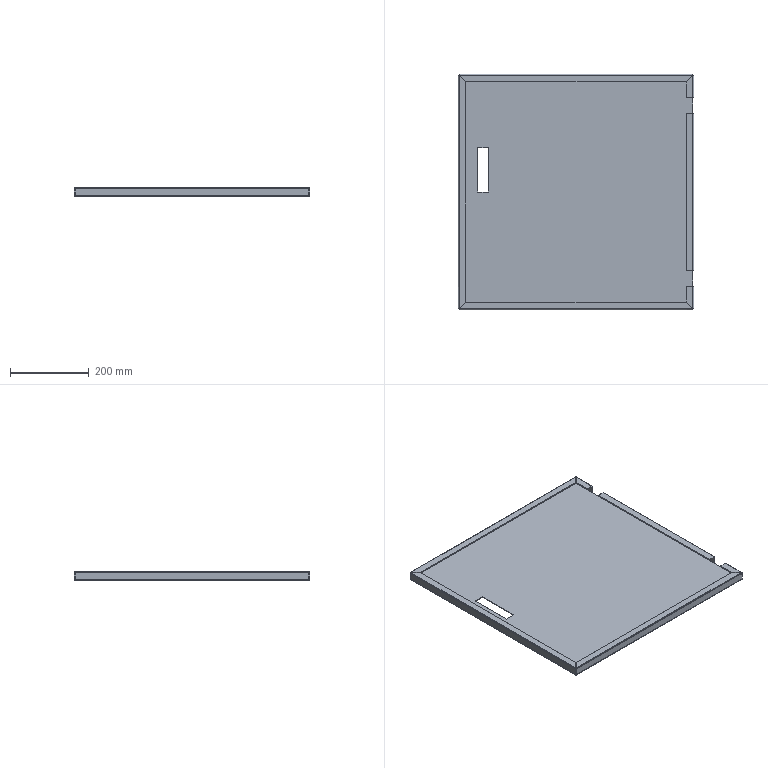Part | SolidWorks | features EdgeFlange 2, ICE 2, FlatPattern 1, SMBaseFlange 1, SheetMetal 1 | 1 solid | 110 faces | box 600 x 600 x 22 mm | volume 660192 mm3 | plane 70 | cylinder 24 | spline 16 | commonest cylinder face diameters 1.473 x12 4.473 x12